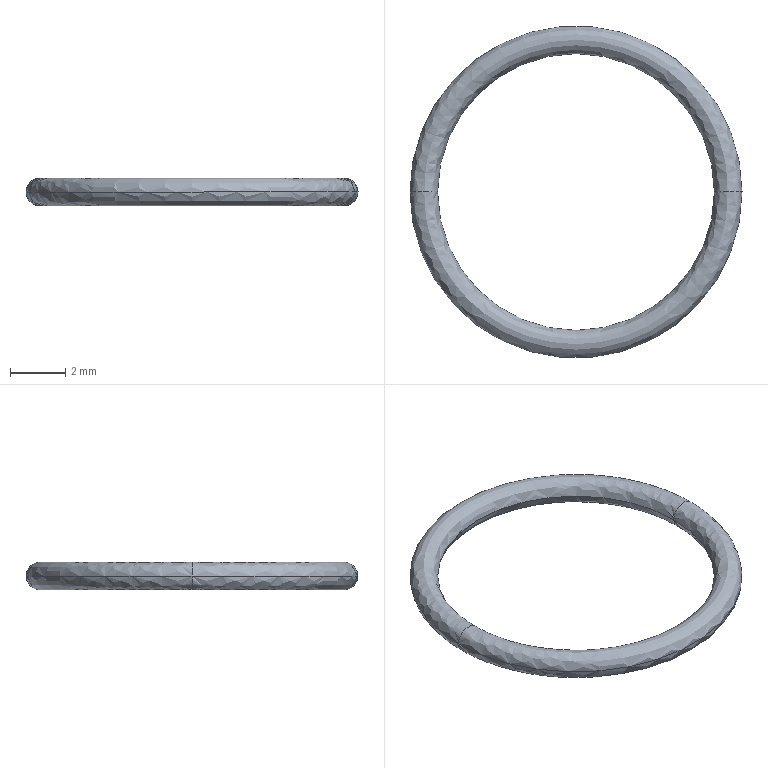Part | SolidWorks | features BaseBody 1 | 1 solid | 4 faces | box 12 x 12 x 1 mm | volume 27.139 mm3 | spline 4
STEP:
#1=CARTESIAN_POINT('',(486.537,37.715,85.866));
#2=VERTEX_POINT('',#1);
#3=CARTESIAN_POINT('',(474.537,37.715,85.866));
#4=VERTEX_POINT('',#3);
#5=CARTESIAN_POINT('',(480.537,37.715,85.866));
#6=DIRECTION('',(0.000000013,0.,-1.));
#7=DIRECTION('',(-1.,0.,-0.000000013));
#8=AXIS2_PLACEMENT_3D('',#5,#6,#7);
#9=CIRCLE('',#8,6.);
#10=EDGE_CURVE('',#2,#4,#9,.T.);
#11=ORIENTED_EDGE('',*,*,#10,.F.);
#12=CARTESIAN_POINT('',(485.537,37.715,85.866));
#13=VERTEX_POINT('',#12);
#14=CARTESIAN_POINT('',(486.537,37.715,85.866));
#15=CARTESIAN_POINT('',(486.537,37.715,85.924));
#16=CARTESIAN_POINT('',(486.515,37.715,86.049));
#17=CARTESIAN_POINT('',(486.412,37.715,86.218));
#18=CARTESIAN_POINT('',(486.241,37.715,86.338));
#19=CARTESIAN_POINT('',(486.037,37.715,86.38));
#20=CARTESIAN_POINT('',(485.833,37.715,86.338));
#21=CARTESIAN_POINT('',(485.662,37.715,86.218));
#22=CARTESIAN_POINT('',(485.559,37.715,86.049));
#23=CARTESIAN_POINT('',(485.537,37.715,85.924));
#24=CARTESIAN_POINT('',(485.537,37.715,85.866));
#25=B_SPLINE_CURVE_WITH_KNOTS('',3,(#14,#15,#16,#17,#18,#19,#20,#21,#22,#23,#24),.UNSPECIFIED.,.F.,.F.,(4,1,1,1,1,1,1,1,4),(0.01923,0.125,0.25,0.375,0.5,0.625,0.75,0.875,0.9808),.UNSPECIFIED.);
#26=EDGE_CURVE('',#2,#13,#25,.T.);
#27=ORIENTED_EDGE('',*,*,#26,.T.);
#28=CARTESIAN_POINT('',(475.537,37.715,85.866));
#29=VERTEX_POINT('',#28);
#30=CARTESIAN_POINT('',(480.537,37.715,85.866));
#31=DIRECTION('',(-0.000000013,0.,1.));
#32=DIRECTION('',(-1.,0.,-0.000000013));
#33=AXIS2_PLACEMENT_3D('',#30,#31,#32);
#34=CIRCLE('',#33,5.);
#35=EDGE_CURVE('',#29,#13,#34,.T.);
#36=ORIENTED_EDGE('',*,*,#35,.F.);
#37=CARTESIAN_POINT('',(474.537,37.715,85.866));
#38=CARTESIAN_POINT('',(474.537,37.715,85.924));
#39=CARTESIAN_POINT('',(474.559,37.715,86.049));
#40=CARTESIAN_POINT('',(474.662,37.715,86.218));
#41=CARTESIAN_POINT('',(474.833,37.715,86.338));
#42=CARTESIAN_POINT('',(475.037,37.715,86.38));
#43=CARTESIAN_POINT('',(475.241,37.715,86.338));
#44=CARTESIAN_POINT('',(475.412,37.715,86.218));
#45=CARTESIAN_POINT('',(475.515,37.715,86.049));
#46=CARTESIAN_POINT('',(475.537,37.715,85.924));
#47=CARTESIAN_POINT('',(475.537,37.715,85.866));
#48=B_SPLINE_CURVE_WITH_KNOTS('',3,(#37,#38,#39,#40,#41,#42,#43,#44,#45,#46,#47),.UNSPECIFIED.,.F.,.F.,(4,1,1,1,1,1,1,1,4),(0.01923,0.125,0.25,0.375,0.5,0.625,0.75,0.875,0.9808),.UNSPECIFIED.);
#49=EDGE_CURVE('',#4,#29,#48,.T.);
#50=ORIENTED_EDGE('',*,*,#49,.F.);
#51=EDGE_LOOP('',(#11,#27,#36,#50));
#52=FACE_OUTER_BOUND('',#51,.T.);
#53=CARTESIAN_POINT('',(474.537,37.715,85.866));
#54=CARTESIAN_POINT('',(474.537,25.715,85.866));
#55=CARTESIAN_POINT('',(486.537,25.715,85.866));
#56=CARTESIAN_POINT('',(486.537,37.715,85.866));
#57=CARTESIAN_POINT('',(474.537,37.715,85.924));
#58=CARTESIAN_POINT('',(474.537,25.715,85.924));
#59=CARTESIAN_POINT('',(486.537,25.715,85.924));
#60=CARTESIAN_POINT('',(486.537,37.715,85.924));
#61=CARTESIAN_POINT('',(474.559,37.715,86.049));
#62=CARTESIAN_POINT('',(474.559,25.758,86.049));
#63=CARTESIAN_POINT('',(486.515,25.758,86.049));
#64=CARTESIAN_POINT('',(486.515,37.715,86.049));
#65=CARTESIAN_POINT('',(474.662,37.715,86.218));
#66=CARTESIAN_POINT('',(474.662,25.965,86.218));
#67=CARTESIAN_POINT('',(486.412,25.965,86.218));
#68=CARTESIAN_POINT('',(486.412,37.715,86.218));
#69=CARTESIAN_POINT('',(474.833,37.715,86.338));
#70=CARTESIAN_POINT('',(474.833,26.306,86.338));
#71=CARTESIAN_POINT('',(486.241,26.306,86.338));
#72=CARTESIAN_POINT('',(486.241,37.715,86.338));
#73=CARTESIAN_POINT('',(475.037,37.715,86.38));
#74=CARTESIAN_POINT('',(475.037,26.715,86.38));
#75=CARTESIAN_POINT('',(486.037,26.715,86.38));
#76=CARTESIAN_POINT('',(486.037,37.715,86.38));
#77=CARTESIAN_POINT('',(475.241,37.715,86.338));
#78=CARTESIAN_POINT('',(475.241,27.123,86.338));
#79=CARTESIAN_POINT('',(485.833,27.123,86.338));
#80=CARTESIAN_POINT('',(485.833,37.715,86.338));
#81=CARTESIAN_POINT('',(475.412,37.715,86.218));
#82=CARTESIAN_POINT('',(475.412,27.464,86.218));
#83=CARTESIAN_POINT('',(485.662,27.464,86.218));
#84=CARTESIAN_POINT('',(485.662,37.715,86.218));
#85=CARTESIAN_POINT('',(475.515,37.715,86.049));
#86=CARTESIAN_POINT('',(475.515,27.671,86.049));
#87=CARTESIAN_POINT('',(485.559,27.671,86.049));
#88=CARTESIAN_POINT('',(485.559,37.715,86.049));
#89=CARTESIAN_POINT('',(475.537,37.715,85.924));
#90=CARTESIAN_POINT('',(475.537,27.715,85.924));
#91=CARTESIAN_POINT('',(485.537,27.715,85.924));
#92=CARTESIAN_POINT('',(485.537,37.715,85.924));
#93=CARTESIAN_POINT('',(475.537,37.715,85.866));
#94=CARTESIAN_POINT('',(475.537,27.715,85.866));
#95=CARTESIAN_POINT('',(485.537,27.715,85.866));
#96=CARTESIAN_POINT('',(485.537,37.715,85.866));
#97=(BOUNDED_SURFACE()B_SPLINE_SURFACE(3,3,((#53,#54,#55,#56),(#57,#58,#59,#60),(#61,#62,#63,#64),(#65,#66,#67,#68),(#69,#70,#71,#72),(#73,#74,#75,#76),(#77,#78,#79,#80),(#81,#82,#83,#84),(#85,#86,#87,#88),(#89,#90,#91,#92),(#93,#94,#95,#96)),.UNSPECIFIED.,.F.,.F.,.T.)B_SPLINE_SURFACE_WITH_KNOTS((4,1,1,1,1,1,1,1,4),(4,4),(0.01923,0.125,0.25,0.375,0.5,0.625,0.75,0.875,0.9808),(0.,1.),.UNSPECIFIED.)GEOMETRIC_REPRESENTATION_ITEM()RATIONAL_B_SPLINE_SURFACE(((1.,0.3333,0.3333,1.),(1.,0.3333,0.3333,1.),(1.,0.3333,0.3333,1.),(1.,0.3333,0.3333,1.),(1.,0.3333,0.3333,1.),(1.,0.3333,0.3333,1.),(1.,0.3333,0.3333,1.),(1.,0.3333,0.3333,1.),(1.,0.3333,0.3333,1.),(1.,0.3333,0.3333,1.),(1.,0.3333,0.3333,1.)))REPRESENTATION_ITEM('')SURFACE());
#98=ADVANCED_FACE('',(#52),#97,.F.);
#99=ORIENTED_EDGE('',*,*,#35,.T.);
#100=CARTESIAN_POINT('',(485.537,37.715,85.866));
#101=CARTESIAN_POINT('',(485.537,37.715,85.808));
#102=CARTESIAN_POINT('',(485.559,37.715,85.683));
#103=CARTESIAN_POINT('',(485.662,37.715,85.514));
#104=CARTESIAN_POINT('',(485.833,37.715,85.394));
#105=CARTESIAN_POINT('',(486.037,37.715,85.352));
#106=CARTESIAN_POINT('',(486.241,37.715,85.394));
#107=CARTESIAN_POINT('',(486.412,37.715,85.514));
#108=CARTESIAN_POINT('',(486.515,37.715,85.683));
#109=CARTESIAN_POINT('',(486.537,37.715,85.808));
#110=CARTESIAN_POINT('',(486.537,37.715,85.866));
#111=B_SPLINE_CURVE_WITH_KNOTS('',3,(#100,#101,#102,#103,#104,#105,#106,#107,#108,#109,#110),.UNSPECIFIED.,.F.,.F.,(4,1,1,1,1,1,1,1,4),(0.01923,0.125,0.25,0.375,0.5,0.625,0.75,0.875,0.9808),.UNSPECIFIED.);
#112=EDGE_CURVE('',#13,#2,#111,.T.);
#113=ORIENTED_EDGE('',*,*,#112,.T.);
#114=ORIENTED_EDGE('',*,*,#10,.T.);
#115=CARTESIAN_POINT('',(475.537,37.715,85.866));
#116=CARTESIAN_POINT('',(475.537,37.715,85.808));
#117=CARTESIAN_POINT('',(475.515,37.715,85.683));
#118=CARTESIAN_POINT('',(475.412,37.715,85.514));
#119=CARTESIAN_POINT('',(475.241,37.715,85.394));
#120=CARTESIAN_POINT('',(475.037,37.715,85.352));
#121=CARTESIAN_POINT('',(474.833,37.715,85.394));
#122=CARTESIAN_POINT('',(474.662,37.715,85.514));
#123=CARTESIAN_POINT('',(474.559,37.715,85.683));
#124=CARTESIAN_POINT('',(474.537,37.715,85.808));
#125=CARTESIAN_POINT('',(474.537,37.715,85.866));
#126=B_SPLINE_CURVE_WITH_KNOTS('',3,(#115,#116,#117,#118,#119,#120,#121,#122,#123,#124,#125),.UNSPECIFIED.,.F.,.F.,(4,1,1,1,1,1,1,1,4),(0.01923,0.125,0.25,0.375,0.5,0.625,0.75,0.875,0.9808),.UNSPECIFIED.);
#127=EDGE_CURVE('',#29,#4,#126,.T.);
#128=ORIENTED_EDGE('',*,*,#127,.F.);
#129=EDGE_LOOP('',(#99,#113,#114,#128));
#130=FACE_OUTER_BOUND('',#129,.T.);
#131=CARTESIAN_POINT('',(475.537,37.715,85.866));
#132=CARTESIAN_POINT('',(475.537,27.715,85.866));
#133=CARTESIAN_POINT('',(485.537,27.715,85.866));
#134=CARTESIAN_POINT('',(485.537,37.715,85.866));
#135=CARTESIAN_POINT('',(475.537,37.715,85.808));
#136=CARTESIAN_POINT('',(475.537,27.715,85.808));
#137=CARTESIAN_POINT('',(485.537,27.715,85.808));
#138=CARTESIAN_POINT('',(485.537,37.715,85.808));
#139=CARTESIAN_POINT('',(475.515,37.715,85.683));
#140=CARTESIAN_POINT('',(475.515,27.671,85.683));
#141=CARTESIAN_POINT('',(485.559,27.671,85.683));
#142=CARTESIAN_POINT('',(485.559,37.715,85.683));
#143=CARTESIAN_POINT('',(475.412,37.715,85.514));
#144=CARTESIAN_POINT('',(475.412,27.464,85.514));
#145=CARTESIAN_POINT('',(485.662,27.464,85.514));
#146=CARTESIAN_POINT('',(485.662,37.715,85.514));
#147=CARTESIAN_POINT('',(475.241,37.715,85.394));
#148=CARTESIAN_POINT('',(475.241,27.123,85.394));
#149=CARTESIAN_POINT('',(485.833,27.123,85.394));
#150=CARTESIAN_POINT('',(485.833,37.715,85.394));
#151=CARTESIAN_POINT('',(475.037,37.715,85.352));
#152=CARTESIAN_POINT('',(475.037,26.715,85.352));
#153=CARTESIAN_POINT('',(486.037,26.715,85.352));
#154=CARTESIAN_POINT('',(486.037,37.715,85.352));
#155=CARTESIAN_POINT('',(474.833,37.715,85.394));
#156=CARTESIAN_POINT('',(474.833,26.306,85.394));
#157=CARTESIAN_POINT('',(486.241,26.306,85.394));
#158=CARTESIAN_POINT('',(486.241,37.715,85.394));
#159=CARTESIAN_POINT('',(474.662,37.715,85.514));
#160=CARTESIAN_POINT('',(474.662,25.965,85.514));
#161=CARTESIAN_POINT('',(486.412,25.965,85.514));
#162=CARTESIAN_POINT('',(486.412,37.715,85.514));
#163=CARTESIAN_POINT('',(474.559,37.715,85.683));
#164=CARTESIAN_POINT('',(474.559,25.758,85.683));
#165=CARTESIAN_POINT('',(486.515,25.758,85.683));
#166=CARTESIAN_POINT('',(486.515,37.715,85.683));
#167=CARTESIAN_POINT('',(474.537,37.715,85.808));
#168=CARTESIAN_POINT('',(474.537,25.715,85.808));
#169=CARTESIAN_POINT('',(486.537,25.715,85.808));
#170=CARTESIAN_POINT('',(486.537,37.715,85.808));
#171=CARTESIAN_POINT('',(474.537,37.715,85.866));
#172=CARTESIAN_POINT('',(474.537,25.715,85.866));
#173=CARTESIAN_POINT('',(486.537,25.715,85.866));
#174=CARTESIAN_POINT('',(486.537,37.715,85.866));
#175=(BOUNDED_SURFACE()B_SPLINE_SURFACE(3,3,((#131,#132,#133,#134),(#135,#136,#137,#138),(#139,#140,#141,#142),(#143,#144,#145,#146),(#147,#148,#149,#150),(#151,#152,#153,#154),(#155,#156,#157,#158),(#159,#160,#161,#162),(#163,#164,#165,#166),(#167,#168,#169,#170),(#171,#172,#173,#174)),.UNSPECIFIED.,.F.,.F.,.T.)B_SPLINE_SURFACE_WITH_KNOTS((4,1,1,1,1,1,1,1,4),(4,4),(0.01923,0.125,0.25,0.375,0.5,0.625,0.75,0.875,0.9808),(0.,1.),.UNSPECIFIED.)GEOMETRIC_REPRESENTATION_ITEM()RATIONAL_B_SPLINE_SURFACE(((1.,0.3333,0.3333,1.),(1.,0.3333,0.3333,1.),(1.,0.3333,0.3333,1.),(1.,0.3333,0.3333,1.),(1.,0.3333,0.3333,1.),(1.,0.3333,0.3333,1.),(1.,0.3333,0.3333,1.),(1.,0.3333,0.3333,1.),(1.,0.3333,0.3333,1.),(1.,0.3333,0.3333,1.),(1.,0.3333,0.3333,1.)))REPRESENTATION_ITEM('')SURFACE());
#176=ADVANCED_FACE('',(#130),#175,.F.);
#177=ORIENTED_EDGE('',*,*,#26,.F.);
#178=CARTESIAN_POINT('',(480.537,37.715,85.866));
#179=DIRECTION('',(0.000000013,0.,-1.));
#180=DIRECTION('',(-1.,0.,-0.000000013));
#181=AXIS2_PLACEMENT_3D('',#178,#179,#180);
#182=CIRCLE('',#181,6.);
#183=EDGE_CURVE('',#4,#2,#182,.T.);
#184=ORIENTED_EDGE('',*,*,#183,.F.);
#185=ORIENTED_EDGE('',*,*,#49,.T.);
#186=CARTESIAN_POINT('',(480.537,37.715,85.866));
#187=DIRECTION('',(-0.000000013,0.,1.));
#188=DIRECTION('',(-1.,0.,-0.000000013));
#189=AXIS2_PLACEMENT_3D('',#186,#187,#188);
#190=CIRCLE('',#189,5.);
#191=EDGE_CURVE('',#13,#29,#190,.T.);
#192=ORIENTED_EDGE('',*,*,#191,.F.);
#193=EDGE_LOOP('',(#177,#184,#185,#192));
#194=FACE_OUTER_BOUND('',#193,.T.);
#195=CARTESIAN_POINT('',(486.537,37.715,85.866));
#196=CARTESIAN_POINT('',(486.537,49.715,85.866));
#197=CARTESIAN_POINT('',(474.537,49.715,85.866));
#198=CARTESIAN_POINT('',(474.537,37.715,85.866));
#199=CARTESIAN_POINT('',(486.537,37.715,85.924));
#200=CARTESIAN_POINT('',(486.537,49.715,85.924));
#201=CARTESIAN_POINT('',(474.537,49.715,85.924));
#202=CARTESIAN_POINT('',(474.537,37.715,85.924));
#203=CARTESIAN_POINT('',(486.515,37.715,86.049));
#204=CARTESIAN_POINT('',(486.515,49.671,86.049));
#205=CARTESIAN_POINT('',(474.559,49.671,86.049));
#206=CARTESIAN_POINT('',(474.559,37.715,86.049));
#207=CARTESIAN_POINT('',(486.412,37.715,86.218));
#208=CARTESIAN_POINT('',(486.412,49.464,86.218));
#209=CARTESIAN_POINT('',(474.662,49.464,86.218));
#210=CARTESIAN_POINT('',(474.662,37.715,86.218));
#211=CARTESIAN_POINT('',(486.241,37.715,86.338));
#212=CARTESIAN_POINT('',(486.241,49.123,86.338));
#213=CARTESIAN_POINT('',(474.833,49.123,86.338));
#214=CARTESIAN_POINT('',(474.833,37.715,86.338));
#215=CARTESIAN_POINT('',(486.037,37.715,86.38));
#216=CARTESIAN_POINT('',(486.037,48.715,86.38));
#217=CARTESIAN_POINT('',(475.037,48.715,86.38));
#218=CARTESIAN_POINT('',(475.037,37.715,86.38));
#219=CARTESIAN_POINT('',(485.833,37.715,86.338));
#220=CARTESIAN_POINT('',(485.833,48.306,86.338));
#221=CARTESIAN_POINT('',(475.241,48.306,86.338));
#222=CARTESIAN_POINT('',(475.241,37.715,86.338));
#223=CARTESIAN_POINT('',(485.662,37.715,86.218));
#224=CARTESIAN_POINT('',(485.662,47.965,86.218));
#225=CARTESIAN_POINT('',(475.412,47.965,86.218));
#226=CARTESIAN_POINT('',(475.412,37.715,86.218));
#227=CARTESIAN_POINT('',(485.559,37.715,86.049));
#228=CARTESIAN_POINT('',(485.559,47.758,86.049));
#229=CARTESIAN_POINT('',(475.515,47.758,86.049));
#230=CARTESIAN_POINT('',(475.515,37.715,86.049));
#231=CARTESIAN_POINT('',(485.537,37.715,85.924));
#232=CARTESIAN_POINT('',(485.537,47.715,85.924));
#233=CARTESIAN_POINT('',(475.537,47.715,85.924));
#234=CARTESIAN_POINT('',(475.537,37.715,85.924));
#235=CARTESIAN_POINT('',(485.537,37.715,85.866));
#236=CARTESIAN_POINT('',(485.537,47.715,85.866));
#237=CARTESIAN_POINT('',(475.537,47.715,85.866));
#238=CARTESIAN_POINT('',(475.537,37.715,85.866));
#239=(BOUNDED_SURFACE()B_SPLINE_SURFACE(3,3,((#195,#196,#197,#198),(#199,#200,#201,#202),(#203,#204,#205,#206),(#207,#208,#209,#210),(#211,#212,#213,#214),(#215,#216,#217,#218),(#219,#220,#221,#222),(#223,#224,#225,#226),(#227,#228,#229,#230),(#231,#232,#233,#234),(#235,#236,#237,#238)),.UNSPECIFIED.,.F.,.F.,.T.)B_SPLINE_SURFACE_WITH_KNOTS((4,1,1,1,1,1,1,1,4),(4,4),(0.01923,0.125,0.25,0.375,0.5,0.625,0.75,0.875,0.9808),(0.,1.),.UNSPECIFIED.)GEOMETRIC_REPRESENTATION_ITEM()RATIONAL_B_SPLINE_SURFACE(((1.,0.3333,0.3333,1.),(1.,0.3333,0.3333,1.),(1.,0.3333,0.3333,1.),(1.,0.3333,0.3333,1.),(1.,0.3333,0.3333,1.),(1.,0.3333,0.3333,1.),(1.,0.3333,0.3333,1.),(1.,0.3333,0.3333,1.),(1.,0.3333,0.3333,1.),(1.,0.3333,0.3333,1.),(1.,0.3333,0.3333,1.)))REPRESENTATION_ITEM('')SURFACE());
#240=ADVANCED_FACE('',(#194),#239,.F.);
#241=ORIENTED_EDGE('',*,*,#112,.F.);
#242=ORIENTED_EDGE('',*,*,#191,.T.);
#243=ORIENTED_EDGE('',*,*,#127,.T.);
#244=ORIENTED_EDGE('',*,*,#183,.T.);
#245=EDGE_LOOP('',(#241,#242,#243,#244));
#246=FACE_OUTER_BOUND('',#245,.T.);
#247=CARTESIAN_POINT('',(485.537,37.715,85.866));
#248=CARTESIAN_POINT('',(485.537,47.715,85.866));
#249=CARTESIAN_POINT('',(475.537,47.715,85.866));
#250=CARTESIAN_POINT('',(475.537,37.715,85.866));
#251=CARTESIAN_POINT('',(485.537,37.715,85.808));
#252=CARTESIAN_POINT('',(485.537,47.715,85.808));
#253=CARTESIAN_POINT('',(475.537,47.715,85.808));
#254=CARTESIAN_POINT('',(475.537,37.715,85.808));
#255=CARTESIAN_POINT('',(485.559,37.715,85.683));
#256=CARTESIAN_POINT('',(485.559,47.758,85.683));
#257=CARTESIAN_POINT('',(475.515,47.758,85.683));
#258=CARTESIAN_POINT('',(475.515,37.715,85.683));
#259=CARTESIAN_POINT('',(485.662,37.715,85.514));
#260=CARTESIAN_POINT('',(485.662,47.965,85.514));
#261=CARTESIAN_POINT('',(475.412,47.965,85.514));
#262=CARTESIAN_POINT('',(475.412,37.715,85.514));
#263=CARTESIAN_POINT('',(485.833,37.715,85.394));
#264=CARTESIAN_POINT('',(485.833,48.306,85.394));
#265=CARTESIAN_POINT('',(475.241,48.306,85.394));
#266=CARTESIAN_POINT('',(475.241,37.715,85.394));
#267=CARTESIAN_POINT('',(486.037,37.715,85.352));
#268=CARTESIAN_POINT('',(486.037,48.715,85.352));
#269=CARTESIAN_POINT('',(475.037,48.715,85.352));
#270=CARTESIAN_POINT('',(475.037,37.715,85.352));
#271=CARTESIAN_POINT('',(486.241,37.715,85.394));
#272=CARTESIAN_POINT('',(486.241,49.123,85.394));
#273=CARTESIAN_POINT('',(474.833,49.123,85.394));
#274=CARTESIAN_POINT('',(474.833,37.715,85.394));
#275=CARTESIAN_POINT('',(486.412,37.715,85.514));
#276=CARTESIAN_POINT('',(486.412,49.464,85.514));
#277=CARTESIAN_POINT('',(474.662,49.464,85.514));
#278=CARTESIAN_POINT('',(474.662,37.715,85.514));
#279=CARTESIAN_POINT('',(486.515,37.715,85.683));
#280=CARTESIAN_POINT('',(486.515,49.671,85.683));
#281=CARTESIAN_POINT('',(474.559,49.671,85.683));
#282=CARTESIAN_POINT('',(474.559,37.715,85.683));
#283=CARTESIAN_POINT('',(486.537,37.715,85.808));
#284=CARTESIAN_POINT('',(486.537,49.715,85.808));
#285=CARTESIAN_POINT('',(474.537,49.715,85.808));
#286=CARTESIAN_POINT('',(474.537,37.715,85.808));
#287=CARTESIAN_POINT('',(486.537,37.715,85.866));
#288=CARTESIAN_POINT('',(486.537,49.715,85.866));
#289=CARTESIAN_POINT('',(474.537,49.715,85.866));
#290=CARTESIAN_POINT('',(474.537,37.715,85.866));
#291=(BOUNDED_SURFACE()B_SPLINE_SURFACE(3,3,((#247,#248,#249,#250),(#251,#252,#253,#254),(#255,#256,#257,#258),(#259,#260,#261,#262),(#263,#264,#265,#266),(#267,#268,#269,#270),(#271,#272,#273,#274),(#275,#276,#277,#278),(#279,#280,#281,#282),(#283,#284,#285,#286),(#287,#288,#289,#290)),.UNSPECIFIED.,.F.,.F.,.T.)B_SPLINE_SURFACE_WITH_KNOTS((4,1,1,1,1,1,1,1,4),(4,4),(0.01923,0.125,0.25,0.375,0.5,0.625,0.75,0.875,0.9808),(0.,1.),.UNSPECIFIED.)GEOMETRIC_REPRESENTATION_ITEM()RATIONAL_B_SPLINE_SURFACE(((1.,0.3333,0.3333,1.),(1.,0.3333,0.3333,1.),(1.,0.3333,0.3333,1.),(1.,0.3333,0.3333,1.),(1.,0.3333,0.3333,1.),(1.,0.3333,0.3333,1.),(1.,0.3333,0.3333,1.),(1.,0.3333,0.3333,1.),(1.,0.3333,0.3333,1.),(1.,0.3333,0.3333,1.),(1.,0.3333,0.3333,1.)))REPRESENTATION_ITEM('')SURFACE());
#292=ADVANCED_FACE('',(#246),#291,.F.);
#293=CLOSED_SHELL('',(#98,#176,#240,#292));
#294=MANIFOLD_SOLID_BREP('',#293);
#295=CARTESIAN_POINT('',(0.,0.,0.));
#296=DIRECTION('',(0.,0.,1.));
#297=DIRECTION('',(1.,0.,0.));
#298=AXIS2_PLACEMENT_3D('',#295,#296,#297);
#299=(LENGTH_UNIT()NAMED_UNIT(*)SI_UNIT(.MILLI.,.METRE.));
#300=UNCERTAINTY_MEASURE_WITH_UNIT(LENGTH_MEASURE(0.00001),#299,'','');
#301=(NAMED_UNIT(*)PLANE_ANGLE_UNIT()SI_UNIT($,.RADIAN.));
#302=(NAMED_UNIT(*)SI_UNIT($,.STERADIAN.)SOLID_ANGLE_UNIT());
#303=(GEOMETRIC_REPRESENTATION_CONTEXT(3)GLOBAL_UNCERTAINTY_ASSIGNED_CONTEXT((#300))GLOBAL_UNIT_ASSIGNED_CONTEXT((#299,#301,#302))REPRESENTATION_CONTEXT('',''));
#304=ADVANCED_BREP_SHAPE_REPRESENTATION('',(#294,#298),#303);